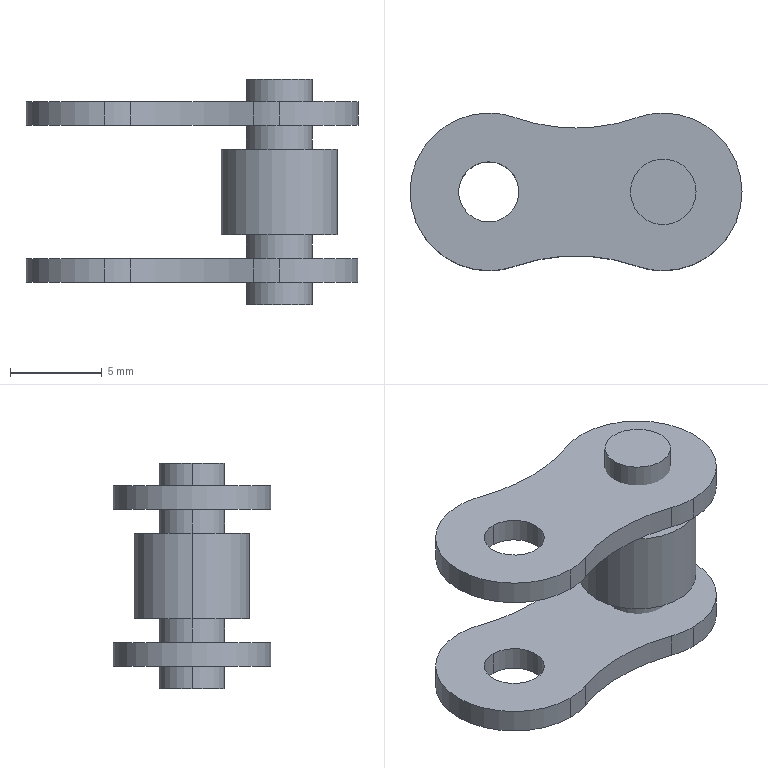Part | STEP file | Industrial chain 06B-1-160 links | 3 solids | 40 faces | box 18.125 x 8.6 x 12.32 mm | volume 522.22 mm3 | cylinder 32 | plane 8 | commonest cylinder face diameters 8.6 x12 3.28 x8 20 x6 3.58 x4 6.35 x2